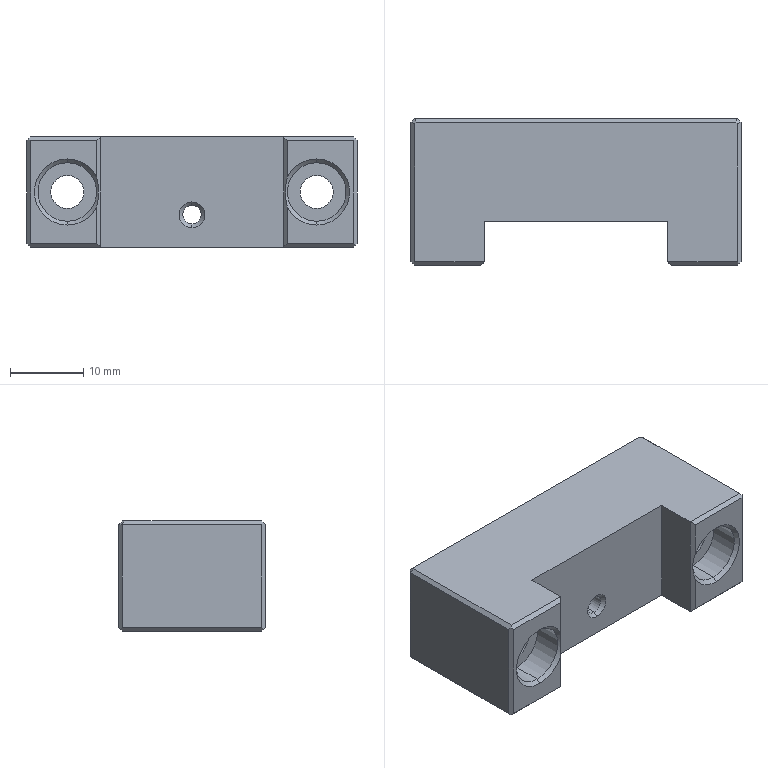Part | SolidWorks | features Chamfer 4, HoleWzd 3, 3DProfileFeature 1, Extrusion 1 | 1 solid | 63 faces | box 45 x 20 x 15 mm | volume 9955 mm3 | plane 31 | cone 18 | cylinder 14 | commonest cylinder face diameters 4 x4 4.5 x4 8 x4 2.5 x2